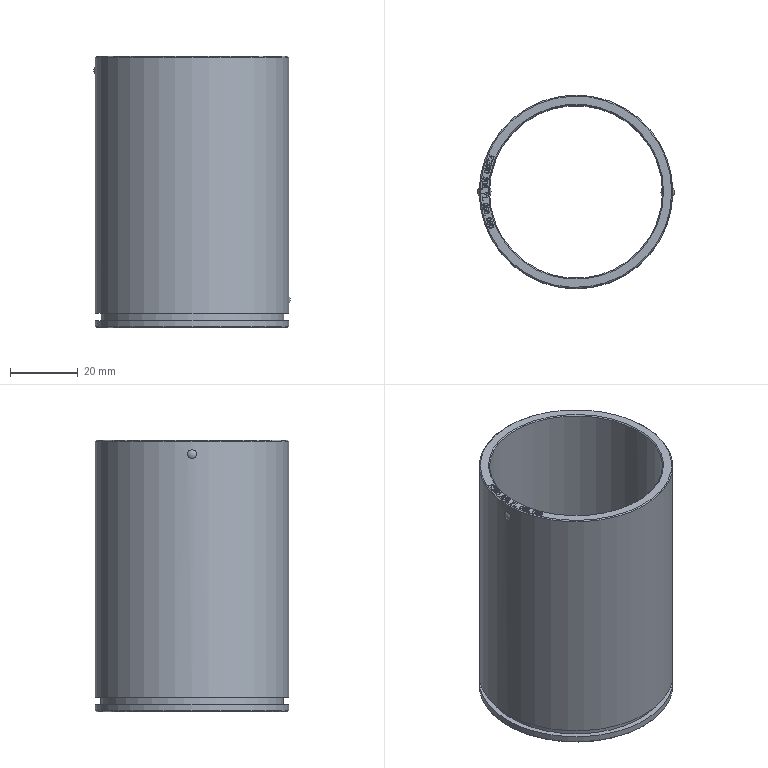Part | NX | features 1 2 | 1 solid | 233 faces | box 58 x 57 x 80 mm | volume 40124 mm3 | spline 138 | plane 83 | cone 4 | cylinder 4 | sphere 4 | commonest cylinder face diameters 57 x2 51 x1 54 x1